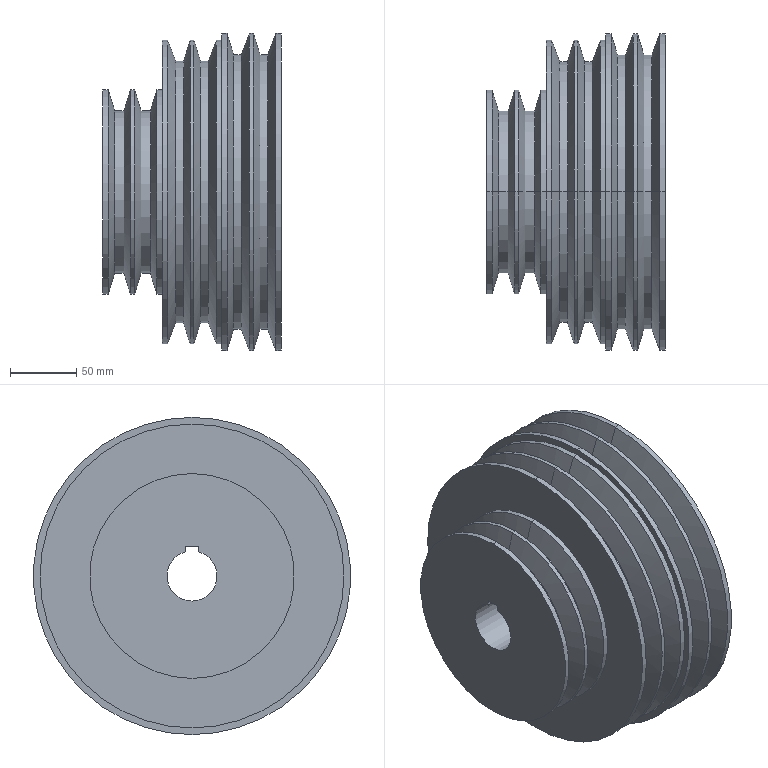Part | SolidWorks | features HoleWzd 1, ICE 1, Revolution 1 | 1 solid | 76 faces | box 135 x 240 x 240 mm | volume 3122246 mm3 | cylinder 39 | cone 28 | plane 9 | commonest cylinder face diameters 155 x6 230 x6 240 x6 8.5 x4 123 x4 198 x4